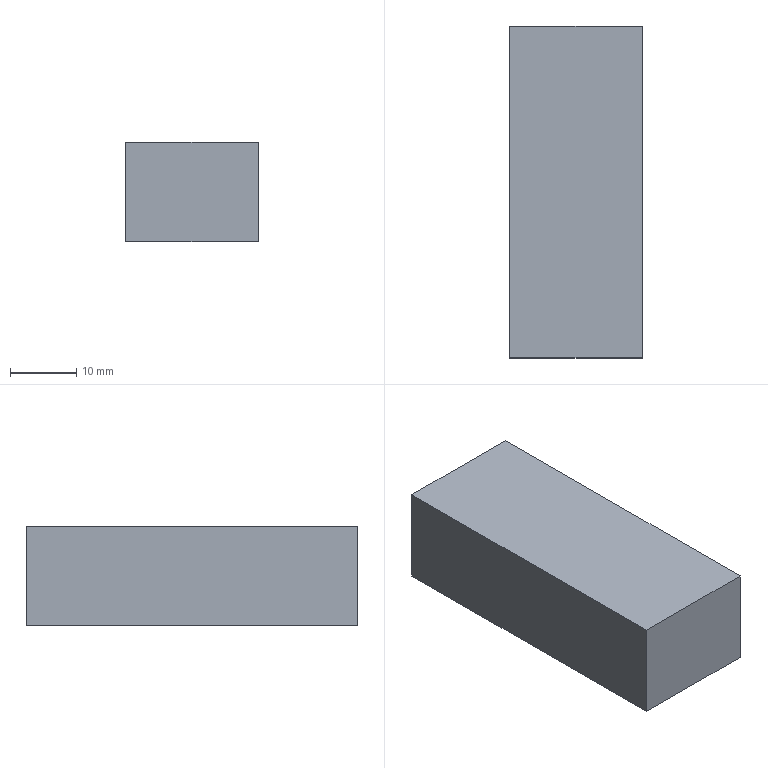Part | SolidWorks | features Extrusion 1 | 1 solid | 6 faces | box 20 x 50 x 15 mm | volume 15000 mm3 | plane 6
STEP:
#1=CARTESIAN_POINT('',(0.,50.,0.));
#2=VERTEX_POINT('',#1);
#3=CARTESIAN_POINT('',(0.,0.,0.));
#4=VERTEX_POINT('',#3);
#5=CARTESIAN_POINT('',(0.,0.,0.));
#6=DIRECTION('',(0.,-1.,0.));
#7=VECTOR('',#6,1000.);
#8=LINE('',#5,#7);
#9=EDGE_CURVE('',#2,#4,#8,.T.);
#10=ORIENTED_EDGE('',*,*,#9,.T.);
#11=CARTESIAN_POINT('',(0.,0.,15.));
#12=VERTEX_POINT('',#11);
#13=CARTESIAN_POINT('',(0.,0.,15.));
#14=DIRECTION('',(0.,0.,-1.));
#15=VECTOR('',#14,1000.);
#16=LINE('',#13,#15);
#17=EDGE_CURVE('',#12,#4,#16,.T.);
#18=ORIENTED_EDGE('',*,*,#17,.F.);
#19=CARTESIAN_POINT('',(0.,50.,15.));
#20=VERTEX_POINT('',#19);
#21=CARTESIAN_POINT('',(0.,0.,15.));
#22=DIRECTION('',(0.,-1.,0.));
#23=VECTOR('',#22,1000.);
#24=LINE('',#21,#23);
#25=EDGE_CURVE('',#20,#12,#24,.T.);
#26=ORIENTED_EDGE('',*,*,#25,.F.);
#27=CARTESIAN_POINT('',(0.,50.,15.));
#28=DIRECTION('',(0.,0.,-1.));
#29=VECTOR('',#28,1000.);
#30=LINE('',#27,#29);
#31=EDGE_CURVE('',#20,#2,#30,.T.);
#32=ORIENTED_EDGE('',*,*,#31,.T.);
#33=EDGE_LOOP('',(#10,#18,#26,#32));
#34=FACE_OUTER_BOUND('',#33,.T.);
#35=CARTESIAN_POINT('',(0.,0.,15.));
#36=DIRECTION('',(1.,0.,0.));
#37=DIRECTION('',(0.,0.,-1.));
#38=AXIS2_PLACEMENT_3D('',#35,#36,#37);
#39=PLANE('',#38);
#40=ADVANCED_FACE('',(#34),#39,.F.);
#41=CARTESIAN_POINT('',(20.,0.,0.));
#42=VERTEX_POINT('',#41);
#43=CARTESIAN_POINT('',(0.,0.,0.));
#44=DIRECTION('',(1.,0.,0.));
#45=VECTOR('',#44,1000.);
#46=LINE('',#43,#45);
#47=EDGE_CURVE('',#4,#42,#46,.T.);
#48=ORIENTED_EDGE('',*,*,#47,.T.);
#49=CARTESIAN_POINT('',(20.,0.,15.));
#50=VERTEX_POINT('',#49);
#51=CARTESIAN_POINT('',(20.,0.,15.));
#52=DIRECTION('',(0.,0.,-1.));
#53=VECTOR('',#52,1000.);
#54=LINE('',#51,#53);
#55=EDGE_CURVE('',#50,#42,#54,.T.);
#56=ORIENTED_EDGE('',*,*,#55,.F.);
#57=CARTESIAN_POINT('',(0.,0.,15.));
#58=DIRECTION('',(1.,0.,0.));
#59=VECTOR('',#58,1000.);
#60=LINE('',#57,#59);
#61=EDGE_CURVE('',#12,#50,#60,.T.);
#62=ORIENTED_EDGE('',*,*,#61,.F.);
#63=ORIENTED_EDGE('',*,*,#17,.T.);
#64=EDGE_LOOP('',(#48,#56,#62,#63));
#65=FACE_OUTER_BOUND('',#64,.T.);
#66=CARTESIAN_POINT('',(0.,0.,15.));
#67=DIRECTION('',(0.,1.,0.));
#68=DIRECTION('',(0.,0.,1.));
#69=AXIS2_PLACEMENT_3D('',#66,#67,#68);
#70=PLANE('',#69);
#71=ADVANCED_FACE('',(#65),#70,.F.);
#72=CARTESIAN_POINT('',(20.,50.,0.));
#73=VERTEX_POINT('',#72);
#74=CARTESIAN_POINT('',(20.,0.,0.));
#75=DIRECTION('',(0.,1.,0.));
#76=VECTOR('',#75,1000.);
#77=LINE('',#74,#76);
#78=EDGE_CURVE('',#42,#73,#77,.T.);
#79=ORIENTED_EDGE('',*,*,#78,.T.);
#80=CARTESIAN_POINT('',(20.,50.,15.));
#81=VERTEX_POINT('',#80);
#82=CARTESIAN_POINT('',(20.,50.,15.));
#83=DIRECTION('',(0.,0.,-1.));
#84=VECTOR('',#83,1000.);
#85=LINE('',#82,#84);
#86=EDGE_CURVE('',#81,#73,#85,.T.);
#87=ORIENTED_EDGE('',*,*,#86,.F.);
#88=CARTESIAN_POINT('',(20.,0.,15.));
#89=DIRECTION('',(0.,1.,0.));
#90=VECTOR('',#89,1000.);
#91=LINE('',#88,#90);
#92=EDGE_CURVE('',#50,#81,#91,.T.);
#93=ORIENTED_EDGE('',*,*,#92,.F.);
#94=ORIENTED_EDGE('',*,*,#55,.T.);
#95=EDGE_LOOP('',(#79,#87,#93,#94));
#96=FACE_OUTER_BOUND('',#95,.T.);
#97=CARTESIAN_POINT('',(20.,0.,15.));
#98=DIRECTION('',(-1.,0.,0.));
#99=DIRECTION('',(0.,0.,1.));
#100=AXIS2_PLACEMENT_3D('',#97,#98,#99);
#101=PLANE('',#100);
#102=ADVANCED_FACE('',(#96),#101,.F.);
#103=CARTESIAN_POINT('',(0.,50.,0.));
#104=DIRECTION('',(-1.,0.,0.));
#105=VECTOR('',#104,1000.);
#106=LINE('',#103,#105);
#107=EDGE_CURVE('',#73,#2,#106,.T.);
#108=ORIENTED_EDGE('',*,*,#107,.T.);
#109=ORIENTED_EDGE('',*,*,#31,.F.);
#110=CARTESIAN_POINT('',(0.,50.,15.));
#111=DIRECTION('',(-1.,0.,0.));
#112=VECTOR('',#111,1000.);
#113=LINE('',#110,#112);
#114=EDGE_CURVE('',#81,#20,#113,.T.);
#115=ORIENTED_EDGE('',*,*,#114,.F.);
#116=ORIENTED_EDGE('',*,*,#86,.T.);
#117=EDGE_LOOP('',(#108,#109,#115,#116));
#118=FACE_OUTER_BOUND('',#117,.T.);
#119=CARTESIAN_POINT('',(0.,50.,15.));
#120=DIRECTION('',(0.,-1.,0.));
#121=DIRECTION('',(0.,0.,-1.));
#122=AXIS2_PLACEMENT_3D('',#119,#120,#121);
#123=PLANE('',#122);
#124=ADVANCED_FACE('',(#118),#123,.F.);
#125=ORIENTED_EDGE('',*,*,#25,.T.);
#126=ORIENTED_EDGE('',*,*,#61,.T.);
#127=ORIENTED_EDGE('',*,*,#92,.T.);
#128=ORIENTED_EDGE('',*,*,#114,.T.);
#129=EDGE_LOOP('',(#125,#126,#127,#128));
#130=FACE_OUTER_BOUND('',#129,.T.);
#131=CARTESIAN_POINT('',(0.,0.,15.));
#132=DIRECTION('',(0.,0.,-1.));
#133=DIRECTION('',(-1.,0.,0.));
#134=AXIS2_PLACEMENT_3D('',#131,#132,#133);
#135=PLANE('',#134);
#136=ADVANCED_FACE('',(#130),#135,.F.);
#137=ORIENTED_EDGE('',*,*,#9,.F.);
#138=ORIENTED_EDGE('',*,*,#107,.F.);
#139=ORIENTED_EDGE('',*,*,#78,.F.);
#140=ORIENTED_EDGE('',*,*,#47,.F.);
#141=EDGE_LOOP('',(#137,#138,#139,#140));
#142=FACE_OUTER_BOUND('',#141,.T.);
#143=CARTESIAN_POINT('',(0.,0.,0.));
#144=DIRECTION('',(0.,0.,-1.));
#145=DIRECTION('',(-1.,0.,0.));
#146=AXIS2_PLACEMENT_3D('',#143,#144,#145);
#147=PLANE('',#146);
#148=ADVANCED_FACE('',(#142),#147,.T.);
#149=CLOSED_SHELL('',(#40,#71,#102,#124,#136,#148));
#150=MANIFOLD_SOLID_BREP('',#149);
#151=CARTESIAN_POINT('',(0.,0.,0.));
#152=DIRECTION('',(0.,0.,1.));
#153=DIRECTION('',(1.,0.,0.));
#154=AXIS2_PLACEMENT_3D('',#151,#152,#153);
#155=(LENGTH_UNIT()NAMED_UNIT(*)SI_UNIT(.MILLI.,.METRE.));
#156=UNCERTAINTY_MEASURE_WITH_UNIT(LENGTH_MEASURE(0.00001),#155,'','');
#157=(NAMED_UNIT(*)PLANE_ANGLE_UNIT()SI_UNIT($,.RADIAN.));
#158=(NAMED_UNIT(*)SI_UNIT($,.STERADIAN.)SOLID_ANGLE_UNIT());
#159=(GEOMETRIC_REPRESENTATION_CONTEXT(3)GLOBAL_UNCERTAINTY_ASSIGNED_CONTEXT((#156))GLOBAL_UNIT_ASSIGNED_CONTEXT((#155,#157,#158))REPRESENTATION_CONTEXT('',''));
#160=ADVANCED_BREP_SHAPE_REPRESENTATION('',(#150,#154),#159);